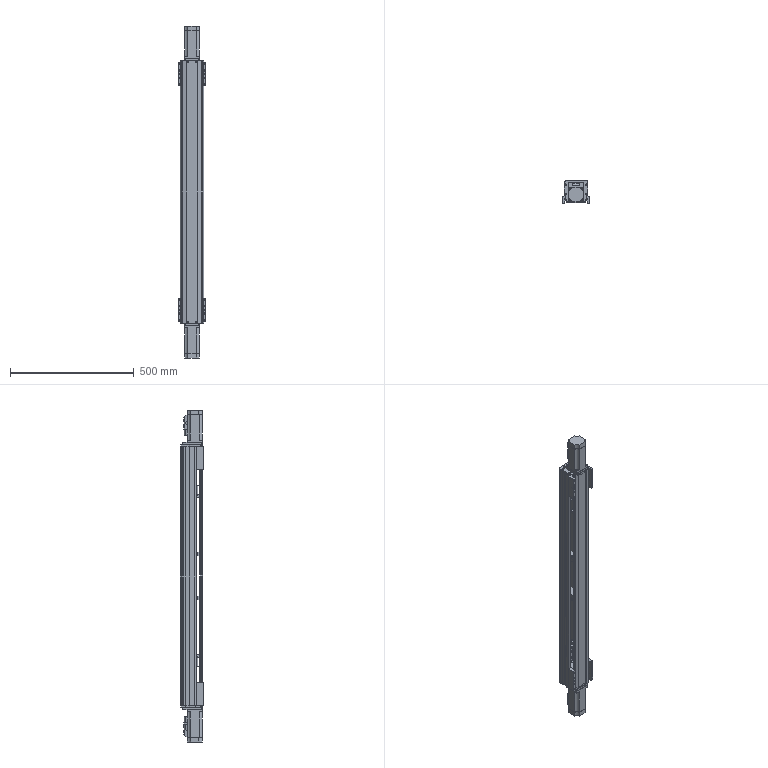Part | NX | 40 solids | 1662 faces | box 110 x 95.023 x 1344 mm | volume 4565293 mm3 | plane 598 | cylinder 452 | torus 334 | sphere 168 | cone 110 | commonest cylinder face diameters 4.5 x48 10 x46 3.3 x34 4.2 x28 2 x24 8 x24